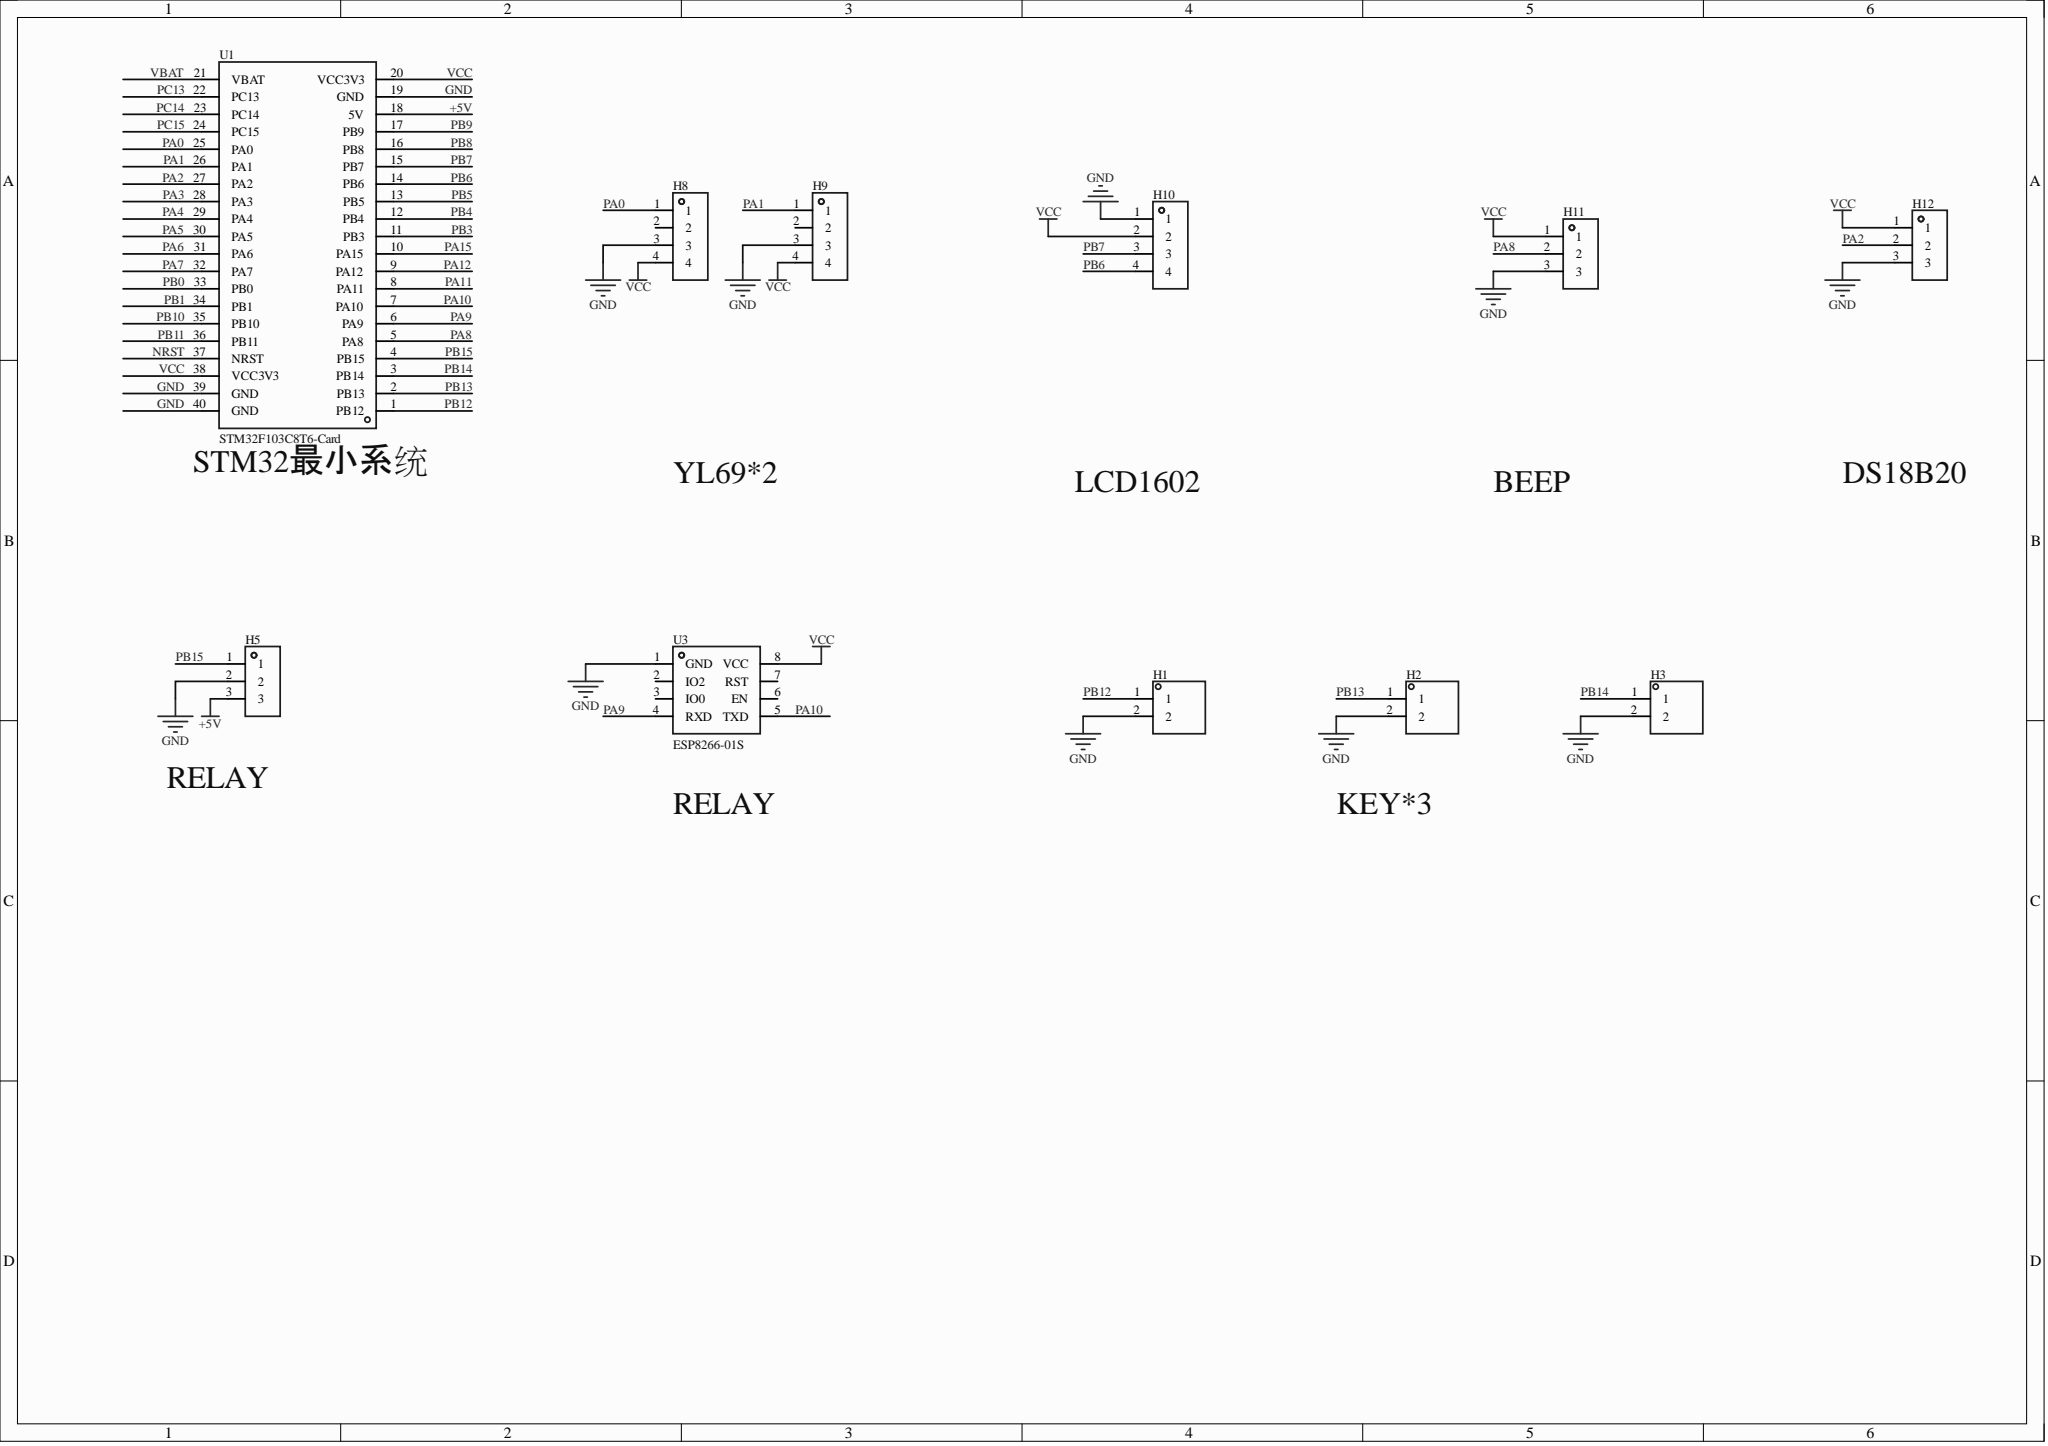Circuit board | Altium Designer | 11 parts | 15 nets
Bill of materials:
Comment,Description,Designator,Footprint,LibRef,Quantity
"","","H1, H2, H3","HDR-TH_2P-P2.54-V-M-1","HDR-M_2.54_1x2P","3"
"","","H5, H11, H12","HDR-TH_3P-P2.54-V-F","HDR-F_2.54_1x3P","3"
"","","H8, H9, H10","HDR-TH_4P-P2.54-V-F","HDR-F_2.54_1x4P","3"
"STM32F103C8T6-Card","","U1","CONN-TH_L53.3-W22.9_STM32F103C8T6-CARD","STM32F103C8T6-Card","1"
"ESP8266-01S","","U3","WIFIM-TH_ESP8266-01S","ESP8266-01S","1"
Netlist (Protel format):
[
H1
HDR-TH_2P-P2.54-V-M-1




]
[
H2
HDR-TH_2P-P2.54-V-M-1




]
[
H3
HDR-TH_2P-P2.54-V-M-1




]
[
H5
HDR-TH_3P-P2.54-V-F




]
[
H8
HDR-TH_4P-P2.54-V-F




]
[
H9
HDR-TH_4P-P2.54-V-F




]
[
H10
HDR-TH_4P-P2.54-V-F




]
[
H11
HDR-TH_3P-P2.54-V-F




]
[
H12
HDR-TH_3P-P2.54-V-F




]
[
U1
CONN-TH_L53.3-W22.9_STM32F103C8T6-CARD
STM32F103C8T6-Card



]
[
U3
WIFIM-TH_ESP8266-01S
ESP8266-01S



]
(
VCC
H8-4
H9-4
H10-2
H11-1
H12-1
U1-20
U1-38
U3-8
)
(
PB15
H5-1
U1-4
)
(
PB14
H3-1
U1-3
)
(
PB13
H2-1
U1-2
)
(
PB12
H1-1
U1-1
)
(
PB7
H10-3
U1-15
)
(
PB6
H10-4
U1-14
)
(
PA10
U1-7
U3-5
)
(
PA9
U1-6
U3-4
)
(
PA8
H11-2
U1-5
)
(
PA2
H12-2
U1-27
)
(
PA1
H9-1
U1-26
)
(
PA0
H8-1
U1-25
)
(
GND
H1-2
H2-2
H3-2
H5-2
H8-3
H9-3
H10-1
H11-3
H12-3
U1-19
U1-39
U1-40
U3-1
)
(
+5V
H5-3
U1-18
)